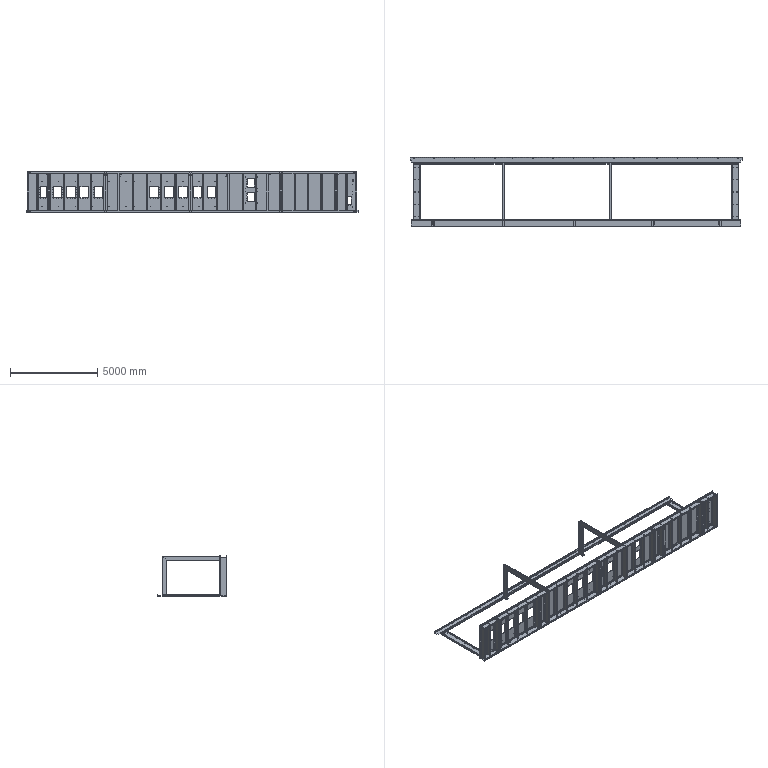Part | STEP file | TS-BASE02_default<by machining> | 99 solids | 2655 faces | box 19000 x 4000 x 2295 mm | volume 1123483782 mm3 | cylinder 1297 | plane 1238 | cone 120 | commonest cylinder face diameters 10 x464 24 x218 21 x120 28 x120 18 x100 26 x58